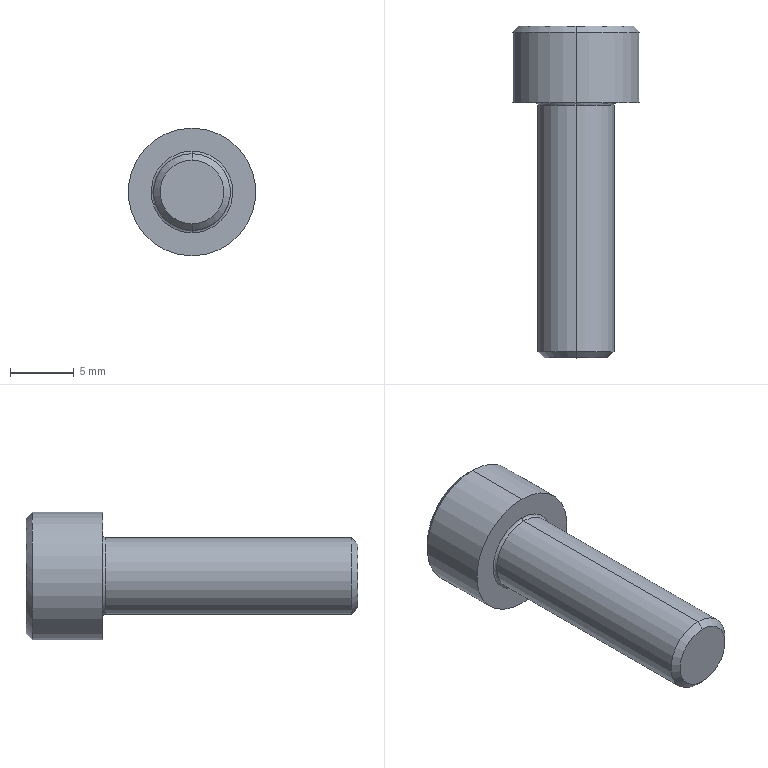Part | STEP file | 1 solid | 20 faces | box 10 x 26 x 10 mm | volume 933.458 mm3 | plane 10 | cone 4 | cylinder 4 | spline 2 | commonest cylinder face diameters 6 x2 10 x2